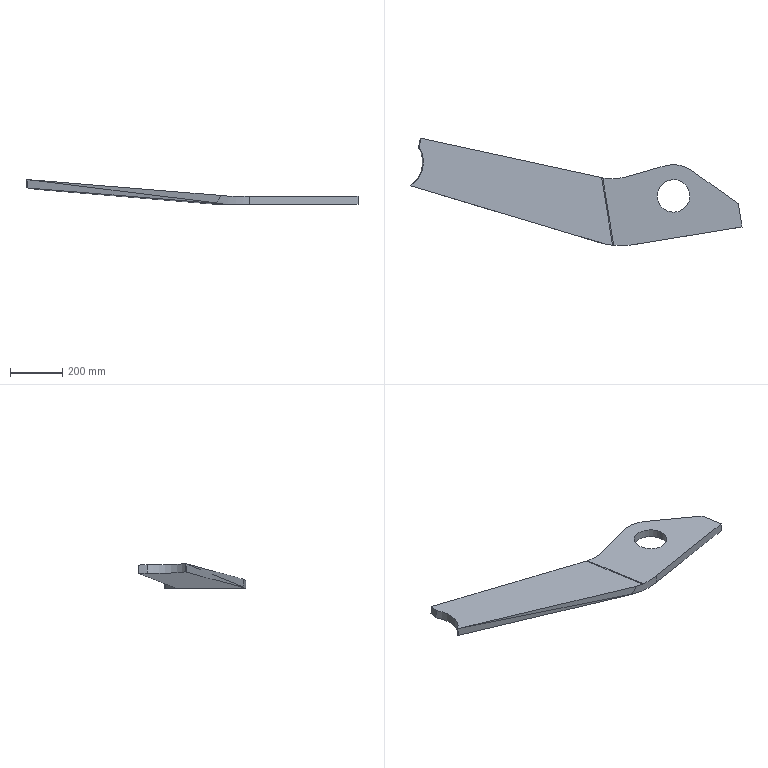Part | SolidWorks | features SplitBody 1 | 1 solid | 24 faces | box 1274 x 411.811 x 95.912 mm | volume 8557362 mm3 | plane 14 | cylinder 9 | spline 1 | commonest cylinder face diameters 125 x2 400 x2 100 x1 164 x1 220 x1 240 x1
STEP:
#1=CARTESIAN_POINT('',(4252.633,293.982,-1052.5));
#2=VERTEX_POINT('',#1);
#3=CARTESIAN_POINT('',(4129.247,273.958,-1052.5));
#4=VERTEX_POINT('',#3);
#5=CARTESIAN_POINT('',(4190.94,283.97,-1052.5));
#6=DIRECTION('',(0.,0.,-1.));
#7=DIRECTION('',(-0.9871,-0.1602,0.));
#8=AXIS2_PLACEMENT_3D('',#5,#6,#7);
#9=CIRCLE('',#8,62.5);
#10=EDGE_CURVE('',#2,#4,#9,.T.);
#11=ORIENTED_EDGE('',*,*,#10,.F.);
#12=CARTESIAN_POINT('',(4252.633,293.982,-1084.5));
#13=VERTEX_POINT('',#12);
#14=CARTESIAN_POINT('',(4252.633,293.982,-1052.5));
#15=DIRECTION('',(0.,0.,-1.));
#16=VECTOR('',#15,1000.);
#17=LINE('',#14,#16);
#18=EDGE_CURVE('',#2,#13,#17,.T.);
#19=ORIENTED_EDGE('',*,*,#18,.T.);
#20=CARTESIAN_POINT('',(4129.247,273.958,-1084.5));
#21=VERTEX_POINT('',#20);
#22=CARTESIAN_POINT('',(4190.94,283.97,-1084.5));
#23=DIRECTION('',(0.,0.,-1.));
#24=DIRECTION('',(-0.9871,-0.1602,0.));
#25=AXIS2_PLACEMENT_3D('',#22,#23,#24);
#26=CIRCLE('',#25,62.5);
#27=EDGE_CURVE('',#13,#21,#26,.T.);
#28=ORIENTED_EDGE('',*,*,#27,.T.);
#29=CARTESIAN_POINT('',(4129.247,273.958,-1052.5));
#30=DIRECTION('',(0.,0.,-1.));
#31=VECTOR('',#30,1000.);
#32=LINE('',#29,#31);
#33=EDGE_CURVE('',#4,#21,#32,.T.);
#34=ORIENTED_EDGE('',*,*,#33,.F.);
#35=EDGE_LOOP('',(#11,#19,#28,#34));
#36=FACE_OUTER_BOUND('',#35,.T.);
#37=CARTESIAN_POINT('',(4190.94,283.97,-1052.5));
#38=DIRECTION('',(0.,0.,-1.));
#39=DIRECTION('',(-0.9871,-0.1602,0.));
#40=AXIS2_PLACEMENT_3D('',#37,#38,#39);
#41=CYLINDRICAL_SURFACE('',#40,62.5);
#42=ADVANCED_FACE('',(#36),#41,.F.);
#43=CARTESIAN_POINT('',(3221.578,504.78,-994.568));
#44=VERTEX_POINT('',#43);
#45=CARTESIAN_POINT('',(3214.351,471.062,-993.471));
#46=VERTEX_POINT('',#45);
#47=CARTESIAN_POINT('',(3221.578,504.78,-994.568));
#48=DIRECTION('',(-0.2095,-0.9773,0.03179));
#49=VECTOR('',#48,1000.);
#50=LINE('',#47,#49);
#51=EDGE_CURVE('',#44,#46,#50,.T.);
#52=ORIENTED_EDGE('',*,*,#51,.T.);
#53=CARTESIAN_POINT('',(3181.855,322.901,-988.588));
#54=VERTEX_POINT('',#53);
#55=CARTESIAN_POINT('',(3120.615,414.189,-984.579));
#56=DIRECTION('',(-0.08603,-0.01396,-0.9962));
#57=DIRECTION('',(-0.9833,-0.1596,0.08716));
#58=AXIS2_PLACEMENT_3D('',#55,#56,#57);
#59=CIRCLE('',#58,110.);
#60=EDGE_CURVE('',#46,#54,#59,.T.);
#61=ORIENTED_EDGE('',*,*,#60,.T.);
#62=CARTESIAN_POINT('',(3927.771,99.208,-1049.87));
#63=VERTEX_POINT('',#62);
#64=CARTESIAN_POINT('',(3181.855,322.901,-988.588));
#65=DIRECTION('',(0.9549,-0.2864,-0.07845));
#66=VECTOR('',#65,1000.);
#67=LINE('',#64,#66);
#68=EDGE_CURVE('',#54,#63,#67,.T.);
#69=ORIENTED_EDGE('',*,*,#68,.T.);
#70=CARTESIAN_POINT('',(3956.763,94.667,-1052.31));
#71=VERTEX_POINT('',#70);
#72=CARTESIAN_POINT('',(3927.771,99.208,-1049.87));
#73=CARTESIAN_POINT('',(3937.357,97.222,-1050.67));
#74=CARTESIAN_POINT('',(3947.029,95.707,-1051.484));
#75=CARTESIAN_POINT('',(3956.763,94.667,-1052.31));
#76=(BOUNDED_CURVE()B_SPLINE_CURVE(3,(#72,#73,#74,#75),.UNSPECIFIED.,.F.,.T.)B_SPLINE_CURVE_WITH_KNOTS((4,4),(1.206,1.303),.UNSPECIFIED.)CURVE()GEOMETRIC_REPRESENTATION_ITEM()RATIONAL_B_SPLINE_CURVE((1.,0.9992,0.9992,1.))REPRESENTATION_ITEM(''));
#77=EDGE_CURVE('',#63,#71,#76,.T.);
#78=ORIENTED_EDGE('',*,*,#77,.T.);
#79=CARTESIAN_POINT('',(3914.616,354.364,-1052.31));
#80=VERTEX_POINT('',#79);
#81=CARTESIAN_POINT('',(3884.78,538.207,-1052.31));
#82=DIRECTION('',(-0.1602,0.9871,0.));
#83=VECTOR('',#82,1000.);
#84=LINE('',#81,#83);
#85=EDGE_CURVE('',#71,#80,#84,.T.);
#86=ORIENTED_EDGE('',*,*,#85,.T.);
#87=CARTESIAN_POINT('',(3914.552,354.378,-1052.304));
#88=VERTEX_POINT('',#87);
#89=CARTESIAN_POINT('',(3956.445,549.838,-1058.662));
#90=DIRECTION('',(-0.08603,-0.01396,-0.9962));
#91=DIRECTION('',(-0.9833,-0.1596,0.08716));
#92=AXIS2_PLACEMENT_3D('',#89,#90,#91);
#93=CIRCLE('',#92,200.);
#94=EDGE_CURVE('',#80,#88,#93,.T.);
#95=ORIENTED_EDGE('',*,*,#94,.T.);
#96=CARTESIAN_POINT('',(3914.552,354.378,-1052.304));
#97=DIRECTION('',(-0.974,0.2114,0.08115));
#98=VECTOR('',#97,1000.);
#99=LINE('',#96,#98);
#100=EDGE_CURVE('',#88,#44,#99,.T.);
#101=ORIENTED_EDGE('',*,*,#100,.T.);
#102=EDGE_LOOP('',(#52,#61,#69,#78,#86,#95,#101));
#103=FACE_OUTER_BOUND('',#102,.T.);
#104=CARTESIAN_POINT('',(3120.615,414.189,-984.579));
#105=DIRECTION('',(0.08603,0.01396,0.9962));
#106=DIRECTION('',(0.9833,0.1596,-0.08716));
#107=AXIS2_PLACEMENT_3D('',#104,#105,#106);
#108=PLANE('',#107);
#109=ADVANCED_FACE('',(#103),#108,.T.);
#110=CARTESIAN_POINT('',(3179.102,322.454,-1020.467));
#111=VERTEX_POINT('',#110);
#112=CARTESIAN_POINT('',(3181.855,322.901,-988.588));
#113=DIRECTION('',(-0.08603,-0.01396,-0.9962));
#114=VECTOR('',#113,1000.);
#115=LINE('',#112,#114);
#116=EDGE_CURVE('',#54,#111,#115,.T.);
#117=ORIENTED_EDGE('',*,*,#116,.F.);
#118=ORIENTED_EDGE('',*,*,#60,.F.);
#119=CARTESIAN_POINT('',(3211.598,470.615,-1025.349));
#120=VERTEX_POINT('',#119);
#121=CARTESIAN_POINT('',(3214.351,471.062,-993.471));
#122=DIRECTION('',(0.08603,0.01396,0.9962));
#123=VECTOR('',#122,1000.);
#124=LINE('',#121,#123);
#125=EDGE_CURVE('',#120,#46,#124,.T.);
#126=ORIENTED_EDGE('',*,*,#125,.F.);
#127=CARTESIAN_POINT('',(3117.862,413.742,-1016.457));
#128=DIRECTION('',(0.08603,0.01396,0.9962));
#129=DIRECTION('',(-0.9833,-0.1596,0.08716));
#130=AXIS2_PLACEMENT_3D('',#127,#128,#129);
#131=CIRCLE('',#130,110.);
#132=EDGE_CURVE('',#111,#120,#131,.T.);
#133=ORIENTED_EDGE('',*,*,#132,.F.);
#134=EDGE_LOOP('',(#117,#118,#126,#133));
#135=FACE_OUTER_BOUND('',#134,.T.);
#136=CARTESIAN_POINT('',(3120.615,414.189,-984.579));
#137=DIRECTION('',(-0.08603,-0.01396,-0.9962));
#138=DIRECTION('',(-0.9833,-0.1596,0.08716));
#139=AXIS2_PLACEMENT_3D('',#136,#137,#138);
#140=CYLINDRICAL_SURFACE('',#139,110.);
#141=ADVANCED_FACE('',(#135),#140,.F.);
#142=ORIENTED_EDGE('',*,*,#125,.T.);
#143=ORIENTED_EDGE('',*,*,#51,.F.);
#144=CARTESIAN_POINT('',(3218.825,504.333,-1026.446));
#145=VERTEX_POINT('',#144);
#146=CARTESIAN_POINT('',(3221.578,504.78,-994.568));
#147=DIRECTION('',(0.08603,0.01396,0.9962));
#148=VECTOR('',#147,1000.);
#149=LINE('',#146,#148);
#150=EDGE_CURVE('',#145,#44,#149,.T.);
#151=ORIENTED_EDGE('',*,*,#150,.F.);
#152=CARTESIAN_POINT('',(3218.825,504.333,-1026.446));
#153=DIRECTION('',(0.2095,0.9773,-0.03179));
#154=VECTOR('',#153,1000.);
#155=LINE('',#152,#154);
#156=EDGE_CURVE('',#120,#145,#155,.T.);
#157=ORIENTED_EDGE('',*,*,#156,.F.);
#158=EDGE_LOOP('',(#142,#143,#151,#157));
#159=FACE_OUTER_BOUND('',#158,.T.);
#160=CARTESIAN_POINT('',(3221.578,504.78,-994.568));
#161=DIRECTION('',(0.974,-0.2114,-0.08115));
#162=DIRECTION('',(0.2095,0.9773,-0.03179));
#163=AXIS2_PLACEMENT_3D('',#160,#161,#162);
#164=PLANE('',#163);
#165=ADVANCED_FACE('',(#159),#164,.F.);
#166=ORIENTED_EDGE('',*,*,#150,.T.);
#167=ORIENTED_EDGE('',*,*,#100,.F.);
#168=CARTESIAN_POINT('',(3911.799,353.931,-1084.183));
#169=VERTEX_POINT('',#168);
#170=CARTESIAN_POINT('',(3914.552,354.378,-1052.304));
#171=DIRECTION('',(0.08603,0.01396,0.9962));
#172=VECTOR('',#171,1000.);
#173=LINE('',#170,#172);
#174=EDGE_CURVE('',#169,#88,#173,.T.);
#175=ORIENTED_EDGE('',*,*,#174,.F.);
#176=CARTESIAN_POINT('',(3218.825,504.333,-1026.446));
#177=DIRECTION('',(0.974,-0.2114,-0.08115));
#178=VECTOR('',#177,1000.);
#179=LINE('',#176,#178);
#180=EDGE_CURVE('',#145,#169,#179,.T.);
#181=ORIENTED_EDGE('',*,*,#180,.F.);
#182=EDGE_LOOP('',(#166,#167,#175,#181));
#183=FACE_OUTER_BOUND('',#182,.T.);
#184=CARTESIAN_POINT('',(3221.578,504.78,-994.568));
#185=DIRECTION('',(-0.2095,-0.9773,0.03179));
#186=DIRECTION('',(0.974,-0.2114,-0.08115));
#187=AXIS2_PLACEMENT_3D('',#184,#185,#186);
#188=PLANE('',#187);
#189=ADVANCED_FACE('',(#183),#188,.F.);
#190=CARTESIAN_POINT('',(3961.25,94.222,-1052.5));
#191=VERTEX_POINT('',#190);
#192=CARTESIAN_POINT('',(3961.25,94.222,-1052.5));
#193=CARTESIAN_POINT('',(3959.751,94.359,-1052.5));
#194=CARTESIAN_POINT('',(3958.255,94.508,-1052.436));
#195=CARTESIAN_POINT('',(3956.763,94.667,-1052.31));
#196=B_SPLINE_CURVE_WITH_KNOTS('',3,(#192,#193,#194,#195),.UNSPECIFIED.,.F.,.F.,(4,4),(0.,0.004513),.UNSPECIFIED.);
#197=EDGE_CURVE('',#191,#71,#196,.T.);
#198=ORIENTED_EDGE('',*,*,#197,.F.);
#199=CARTESIAN_POINT('',(3919.263,352.938,-1052.5));
#200=VERTEX_POINT('',#199);
#201=CARTESIAN_POINT('',(3983.96,-45.707,-1052.5));
#202=DIRECTION('',(0.1602,-0.9871,0.));
#203=VECTOR('',#202,1000.);
#204=LINE('',#201,#203);
#205=EDGE_CURVE('',#200,#191,#204,.T.);
#206=ORIENTED_EDGE('',*,*,#205,.F.);
#207=CARTESIAN_POINT('',(3914.616,354.364,-1052.31));
#208=CARTESIAN_POINT('',(3916.162,353.888,-1052.436));
#209=CARTESIAN_POINT('',(3917.712,353.413,-1052.5));
#210=CARTESIAN_POINT('',(3919.263,352.938,-1052.5));
#211=B_SPLINE_CURVE_WITH_KNOTS('',3,(#207,#208,#209,#210),.UNSPECIFIED.,.F.,.F.,(4,4),(0.,1.),.UNSPECIFIED.);
#212=EDGE_CURVE('',#80,#200,#211,.T.);
#213=ORIENTED_EDGE('',*,*,#212,.F.);
#214=ORIENTED_EDGE('',*,*,#85,.F.);
#215=EDGE_LOOP('',(#198,#206,#213,#214));
#216=FACE_OUTER_BOUND('',#215,.T.);
#217=CARTESIAN_POINT('',(3983.96,-45.707,-1002.5));
#218=DIRECTION('',(-0.1602,0.9871,0.));
#219=DIRECTION('',(0.08603,0.01396,0.9962));
#220=AXIS2_PLACEMENT_3D('',#217,#218,#219);
#221=CYLINDRICAL_SURFACE('',#220,50.);
#222=ADVANCED_FACE('',(#216),#221,.F.);
#223=ORIENTED_EDGE('',*,*,#197,.T.);
#224=ORIENTED_EDGE('',*,*,#77,.F.);
#225=CARTESIAN_POINT('',(3902.027,105.743,-1077.67));
#226=VERTEX_POINT('',#225);
#227=CARTESIAN_POINT('',(3927.771,99.208,-1049.87));
#228=CARTESIAN_POINT('',(3919.096,101.006,-1069.446));
#229=CARTESIAN_POINT('',(3910.509,103.185,-1078.719));
#230=CARTESIAN_POINT('',(3902.027,105.743,-1077.67));
#231=(BOUNDED_CURVE()B_SPLINE_CURVE(3,(#227,#228,#229,#230),.UNSPECIFIED.,.F.,.T.)B_SPLINE_CURVE_WITH_KNOTS((4,4),(3.058,3.146),.UNSPECIFIED.)CURVE()GEOMETRIC_REPRESENTATION_ITEM()RATIONAL_B_SPLINE_CURVE((1.,0.9993,0.9993,1.))REPRESENTATION_ITEM(''));
#232=EDGE_CURVE('',#63,#226,#231,.T.);
#233=ORIENTED_EDGE('',*,*,#232,.T.);
#234=CARTESIAN_POINT('',(3902.027,105.743,-1079.86));
#235=VERTEX_POINT('',#234);
#236=CARTESIAN_POINT('',(3902.027,105.743,-1128.053));
#237=DIRECTION('',(0.,0.,-1.));
#238=VECTOR('',#237,1000.);
#239=LINE('',#236,#238);
#240=EDGE_CURVE('',#226,#235,#239,.T.);
#241=ORIENTED_EDGE('',*,*,#240,.T.);
#242=CARTESIAN_POINT('',(3953.886,94.989,-1084.188));
#243=VERTEX_POINT('',#242);
#244=CARTESIAN_POINT('',(3902.027,105.743,-1079.86));
#245=CARTESIAN_POINT('',(3918.974,100.633,-1081.252));
#246=CARTESIAN_POINT('',(3936.305,97.039,-1082.698));
#247=CARTESIAN_POINT('',(3953.886,94.989,-1084.188));
#248=(BOUNDED_CURVE()B_SPLINE_CURVE(3,(#244,#245,#246,#247),.UNSPECIFIED.,.F.,.T.)B_SPLINE_CURVE_WITH_KNOTS((4,4),(1.117,1.294),.UNSPECIFIED.)CURVE()GEOMETRIC_REPRESENTATION_ITEM()RATIONAL_B_SPLINE_CURVE((1.,0.9974,0.9974,1.))REPRESENTATION_ITEM(''));
#249=EDGE_CURVE('',#235,#243,#248,.T.);
#250=ORIENTED_EDGE('',*,*,#249,.T.);
#251=CARTESIAN_POINT('',(3961.25,94.222,-1084.5));
#252=VERTEX_POINT('',#251);
#253=CARTESIAN_POINT('',(3953.886,94.989,-1084.188));
#254=CARTESIAN_POINT('',(3956.333,94.703,-1084.395));
#255=CARTESIAN_POINT('',(3958.788,94.447,-1084.5));
#256=CARTESIAN_POINT('',(3961.25,94.222,-1084.5));
#257=B_SPLINE_CURVE_WITH_KNOTS('',3,(#253,#254,#255,#256),.UNSPECIFIED.,.F.,.F.,(4,4),(0.,0.007411),.UNSPECIFIED.);
#258=EDGE_CURVE('',#243,#252,#257,.T.);
#259=ORIENTED_EDGE('',*,*,#258,.T.);
#260=CARTESIAN_POINT('',(4036.695,96.844,-1084.5));
#261=VERTEX_POINT('',#260);
#262=CARTESIAN_POINT('',(3988.636,392.969,-1084.5));
#263=DIRECTION('',(0.,0.,1.));
#264=DIRECTION('',(0.9871,0.1602,0.));
#265=AXIS2_PLACEMENT_3D('',#262,#263,#264);
#266=CIRCLE('',#265,300.);
#267=EDGE_CURVE('',#252,#261,#266,.T.);
#268=ORIENTED_EDGE('',*,*,#267,.T.);
#269=CARTESIAN_POINT('',(4036.695,96.844,-1052.5));
#270=VERTEX_POINT('',#269);
#271=CARTESIAN_POINT('',(4036.695,96.844,-1128.053));
#272=DIRECTION('',(0.,0.,1.));
#273=VECTOR('',#272,1000.);
#274=LINE('',#271,#273);
#275=EDGE_CURVE('',#261,#270,#274,.T.);
#276=ORIENTED_EDGE('',*,*,#275,.T.);
#277=CARTESIAN_POINT('',(3988.636,392.969,-1052.5));
#278=DIRECTION('',(0.,0.,-1.));
#279=DIRECTION('',(0.9871,0.1602,0.));
#280=AXIS2_PLACEMENT_3D('',#277,#278,#279);
#281=CIRCLE('',#280,300.);
#282=EDGE_CURVE('',#270,#191,#281,.T.);
#283=ORIENTED_EDGE('',*,*,#282,.T.);
#284=EDGE_LOOP('',(#223,#224,#233,#241,#250,#259,#268,#276,#283));
#285=FACE_OUTER_BOUND('',#284,.T.);
#286=CARTESIAN_POINT('',(3988.636,392.969,-1128.053));
#287=DIRECTION('',(0.,0.,1.));
#288=DIRECTION('',(0.9871,0.1602,0.));
#289=AXIS2_PLACEMENT_3D('',#286,#287,#288);
#290=CYLINDRICAL_SURFACE('',#289,300.);
#291=ADVANCED_FACE('',(#285),#290,.T.);
#292=ORIENTED_EDGE('',*,*,#68,.F.);
#293=CARTESIAN_POINT('',(3902.027,105.743,-1077.67));
#294=DIRECTION('',(-0.9508,0.2867,0.1176));
#295=VECTOR('',#294,1000.);
#296=LINE('',#293,#295);
#297=EDGE_CURVE('',#226,#54,#296,.T.);
#298=ORIENTED_EDGE('',*,*,#297,.F.);
#299=ORIENTED_EDGE('',*,*,#232,.F.);
#300=EDGE_LOOP('',(#292,#298,#299));
#301=FACE_OUTER_BOUND('',#300,.T.);
#302=CARTESIAN_POINT('',(3181.855,322.901,-988.588));
#303=DIRECTION('',(0.2842,0.958,-0.03797));
#304=DIRECTION('',(-0.9549,0.2864,0.07845));
#305=AXIS2_PLACEMENT_3D('',#302,#303,#304);
#306=PLANE('',#305);
#307=ADVANCED_FACE('',(#301),#306,.F.);
#308=CARTESIAN_POINT('',(3181.855,322.901,-1020.711));
#309=VERTEX_POINT('',#308);
#310=CARTESIAN_POINT('',(3181.855,322.901,-1020.711));
#311=DIRECTION('',(0.9545,-0.2878,-0.07839));
#312=VECTOR('',#311,1000.);
#313=LINE('',#310,#312);
#314=EDGE_CURVE('',#309,#235,#313,.T.);
#315=ORIENTED_EDGE('',*,*,#314,.F.);
#316=CARTESIAN_POINT('',(3186.707,320.173,-1021.091));
#317=VERTEX_POINT('',#316);
#318=CARTESIAN_POINT('',(3186.707,320.173,-1021.091));
#319=DIRECTION('',(-0.8697,0.4889,0.06825));
#320=VECTOR('',#319,1000.);
#321=LINE('',#318,#320);
#322=EDGE_CURVE('',#317,#309,#321,.T.);
#323=ORIENTED_EDGE('',*,*,#322,.F.);
#324=CARTESIAN_POINT('',(3179.102,322.454,-1020.467));
#325=DIRECTION('',(0.9549,-0.2864,-0.07845));
#326=VECTOR('',#325,1000.);
#327=LINE('',#324,#326);
#328=EDGE_CURVE('',#111,#317,#327,.T.);
#329=ORIENTED_EDGE('',*,*,#328,.F.);
#330=ORIENTED_EDGE('',*,*,#132,.T.);
#331=ORIENTED_EDGE('',*,*,#156,.T.);
#332=ORIENTED_EDGE('',*,*,#180,.T.);
#333=CARTESIAN_POINT('',(3911.863,353.917,-1084.188));
#334=VERTEX_POINT('',#333);
#335=CARTESIAN_POINT('',(3911.863,353.917,-1084.188));
#336=DIRECTION('',(-0.9741,0.2112,0.08116));
#337=VECTOR('',#336,1000.);
#338=LINE('',#335,#337);
#339=EDGE_CURVE('',#334,#169,#338,.T.);
#340=ORIENTED_EDGE('',*,*,#339,.F.);
#341=CARTESIAN_POINT('',(3882.027,537.761,-1084.188));
#342=DIRECTION('',(-0.1602,0.9871,0.));
#343=VECTOR('',#342,1000.);
#344=LINE('',#341,#343);
#345=EDGE_CURVE('',#243,#334,#344,.T.);
#346=ORIENTED_EDGE('',*,*,#345,.F.);
#347=ORIENTED_EDGE('',*,*,#249,.F.);
#348=EDGE_LOOP('',(#315,#323,#329,#330,#331,#332,#340,#346,#347));
#349=FACE_OUTER_BOUND('',#348,.T.);
#350=CARTESIAN_POINT('',(3117.862,413.742,-1016.457));
#351=DIRECTION('',(0.08603,0.01396,0.9962));
#352=DIRECTION('',(0.9833,0.1596,-0.08716));
#353=AXIS2_PLACEMENT_3D('',#350,#351,#352);
#354=PLANE('',#353);
#355=ADVANCED_FACE('',(#349),#354,.F.);
#356=CARTESIAN_POINT('',(3181.855,322.901,-988.588));
#357=DIRECTION('',(0.1471,-0.08271,-0.9857));
#358=VECTOR('',#357,1000.);
#359=LINE('',#356,#358);
#360=EDGE_CURVE('',#54,#317,#359,.T.);
#361=ORIENTED_EDGE('',*,*,#360,.F.);
#362=ORIENTED_EDGE('',*,*,#116,.T.);
#363=ORIENTED_EDGE('',*,*,#328,.T.);
#364=EDGE_LOOP('',(#361,#362,#363));
#365=FACE_OUTER_BOUND('',#364,.T.);
#366=CARTESIAN_POINT('',(3181.855,322.901,-988.588));
#367=DIRECTION('',(0.2842,0.958,-0.03797));
#368=DIRECTION('',(-0.9549,0.2864,0.07845));
#369=AXIS2_PLACEMENT_3D('',#366,#367,#368);
#370=PLANE('',#369);
#371=ADVANCED_FACE('',(#365),#370,.F.);
#372=CARTESIAN_POINT('',(3914.616,354.364,-1052.31));
#373=DIRECTION('',(0.08603,0.01396,0.9962));
#374=VECTOR('',#373,1000.);
#375=LINE('',#372,#374);
#376=EDGE_CURVE('',#334,#80,#375,.T.);
#377=ORIENTED_EDGE('',*,*,#376,.F.);
#378=ORIENTED_EDGE('',*,*,#339,.T.);
#379=ORIENTED_EDGE('',*,*,#174,.T.);
#380=ORIENTED_EDGE('',*,*,#94,.F.);
#381=EDGE_LOOP('',(#377,#378,#379,#380));
#382=FACE_OUTER_BOUND('',#381,.T.);
#383=CARTESIAN_POINT('',(3956.445,549.838,-1058.662));
#384=DIRECTION('',(-0.08603,-0.01396,-0.9962));
#385=DIRECTION('',(-0.9833,-0.1596,0.08716));
#386=AXIS2_PLACEMENT_3D('',#383,#384,#385);
#387=CYLINDRICAL_SURFACE('',#386,200.);
#388=ADVANCED_FACE('',(#382),#387,.F.);
#389=CARTESIAN_POINT('',(4158.117,399.394,-1052.5));
#390=VERTEX_POINT('',#389);
#391=CARTESIAN_POINT('',(4010.04,357.285,-1052.5));
#392=VERTEX_POINT('',#391);
#393=CARTESIAN_POINT('',(4158.117,399.394,-1052.5));
#394=DIRECTION('',(-0.9619,-0.2735,0.));
#395=VECTOR('',#394,1000.);
#396=LINE('',#393,#395);
#397=EDGE_CURVE('',#390,#392,#396,.T.);
#398=ORIENTED_EDGE('',*,*,#397,.T.);
#399=CARTESIAN_POINT('',(3955.335,549.658,-1052.5));
#400=DIRECTION('',(0.,0.,-1.));
#401=DIRECTION('',(-0.9871,-0.1602,0.));
#402=AXIS2_PLACEMENT_3D('',#399,#400,#401);
#403=CIRCLE('',#402,200.);
#404=EDGE_CURVE('',#392,#200,#403,.T.);
#405=ORIENTED_EDGE('',*,*,#404,.T.);
#406=ORIENTED_EDGE('',*,*,#205,.T.);
#407=ORIENTED_EDGE('',*,*,#282,.F.);
#408=CARTESIAN_POINT('',(4453.472,164.483,-1052.5));
#409=VERTEX_POINT('',#408);
#410=CARTESIAN_POINT('',(3190.003,-40.568,-1052.5));
#411=DIRECTION('',(0.9871,0.1602,0.));
#412=VECTOR('',#411,1000.);
#413=LINE('',#410,#412);
#414=EDGE_CURVE('',#270,#409,#413,.T.);
#415=ORIENTED_EDGE('',*,*,#414,.T.);
#416=CARTESIAN_POINT('',(4439.054,253.321,-1052.5));
#417=VERTEX_POINT('',#416);
#418=CARTESIAN_POINT('',(4379.781,618.543,-1052.5));
#419=DIRECTION('',(-0.1602,0.9871,0.));
#420=VECTOR('',#419,1000.);
#421=LINE('',#418,#420);
#422=EDGE_CURVE('',#409,#417,#421,.T.);
#423=ORIENTED_EDGE('',*,*,#422,.T.);
#424=CARTESIAN_POINT('',(4261.011,381.386,-1052.5));
#425=VERTEX_POINT('',#424);
#426=CARTESIAN_POINT('',(4439.054,253.321,-1052.5));
#427=DIRECTION('',(-0.8118,0.5839,0.));
#428=VECTOR('',#427,1000.);
#429=LINE('',#426,#428);
#430=EDGE_CURVE('',#417,#425,#429,.T.);
#431=ORIENTED_EDGE('',*,*,#430,.T.);
#432=CARTESIAN_POINT('',(4190.94,283.97,-1052.5));
#433=DIRECTION('',(0.,0.,1.));
#434=DIRECTION('',(-0.9871,-0.1602,0.));
#435=AXIS2_PLACEMENT_3D('',#432,#433,#434);
#436=CIRCLE('',#435,120.);
#437=EDGE_CURVE('',#425,#390,#436,.T.);
#438=ORIENTED_EDGE('',*,*,#437,.T.);
#439=EDGE_LOOP('',(#398,#405,#406,#407,#415,#423,#431,#438));
#440=FACE_OUTER_BOUND('',#439,.T.);
#441=CARTESIAN_POINT('',(4190.94,283.97,-1052.5));
#442=DIRECTION('',(0.,0.,-1.));
#443=DIRECTION('',(-0.9871,-0.1602,0.));
#444=AXIS2_PLACEMENT_3D('',#441,#442,#443);
#445=CIRCLE('',#444,62.5);
#446=EDGE_CURVE('',#4,#2,#445,.T.);
#447=ORIENTED_EDGE('',*,*,#446,.T.);
#448=ORIENTED_EDGE('',*,*,#10,.T.);
#449=EDGE_LOOP('',(#447,#448));
#450=FACE_BOUND('',#449,.T.);
#451=CARTESIAN_POINT('',(3116.313,413.491,-1052.5));
#452=DIRECTION('',(0.,0.,1.));
#453=DIRECTION('',(0.9871,0.1602,0.));
#454=AXIS2_PLACEMENT_3D('',#451,#452,#453);
#455=PLANE('',#454);
#456=ADVANCED_FACE('',(#440,#450),#455,.T.);
#457=CARTESIAN_POINT('',(3919.263,352.938,-1084.5));
#458=VERTEX_POINT('',#457);
#459=CARTESIAN_POINT('',(3911.863,353.917,-1084.188));
#460=CARTESIAN_POINT('',(3914.324,353.59,-1084.396));
#461=CARTESIAN_POINT('',(3916.793,353.264,-1084.5));
#462=CARTESIAN_POINT('',(3919.263,352.938,-1084.5));
#463=B_SPLINE_CURVE_WITH_KNOTS('',3,(#459,#460,#461,#462),.UNSPECIFIED.,.F.,.F.,(4,4),(0.,1.),.UNSPECIFIED.);
#464=EDGE_CURVE('',#334,#458,#463,.T.);
#465=ORIENTED_EDGE('',*,*,#464,.F.);
#466=ORIENTED_EDGE('',*,*,#376,.T.);
#467=ORIENTED_EDGE('',*,*,#212,.T.);
#468=CARTESIAN_POINT('',(3919.263,352.938,-1068.5));
#469=DIRECTION('',(0.,0.,1.));
#470=VECTOR('',#469,1000.);
#471=LINE('',#468,#470);
#472=EDGE_CURVE('',#458,#200,#471,.T.);
#473=ORIENTED_EDGE('',*,*,#472,.F.);
#474=EDGE_LOOP('',(#465,#466,#467,#473));
#475=FACE_OUTER_BOUND('',#474,.T.);
#476=CARTESIAN_POINT('',(3919.263,352.938,-1084.82));
#477=CARTESIAN_POINT('',(3916.784,353.262,-1084.82));
#478=CARTESIAN_POINT('',(3914.306,353.587,-1084.715));
#479=CARTESIAN_POINT('',(3911.836,353.913,-1084.507));
#480=CARTESIAN_POINT('',(3919.263,352.938,-1084.5));
#481=CARTESIAN_POINT('',(3916.793,353.264,-1084.5));
#482=CARTESIAN_POINT('',(3914.324,353.59,-1084.396));
#483=CARTESIAN_POINT('',(3911.863,353.917,-1084.188));
#484=CARTESIAN_POINT('',(3919.263,352.938,-1052.5));
#485=CARTESIAN_POINT('',(3917.712,353.413,-1052.5));
#486=CARTESIAN_POINT('',(3916.162,353.888,-1052.436));
#487=CARTESIAN_POINT('',(3914.616,354.364,-1052.31));
#488=B_SPLINE_SURFACE_WITH_KNOTS('',1,3,((#476,#477,#478,#479),(#480,#481,#482,#483),(#484,#485,#486,#487)),.UNSPECIFIED.,.F.,.F.,.F.,(2,1,2),(4,4),(-0.01,0.,1.),(0.,1.),.UNSPECIFIED.);
#489=ADVANCED_FACE('',(#475),#488,.F.);
#490=CARTESIAN_POINT('',(4453.472,164.483,-1084.5));
#491=VERTEX_POINT('',#490);
#492=CARTESIAN_POINT('',(4453.472,164.483,-1084.5));
#493=DIRECTION('',(-0.9871,-0.1602,0.));
#494=VECTOR('',#493,1000.);
#495=LINE('',#492,#494);
#496=EDGE_CURVE('',#491,#261,#495,.T.);
#497=ORIENTED_EDGE('',*,*,#496,.F.);
#498=CARTESIAN_POINT('',(4453.472,164.483,-1052.5));
#499=DIRECTION('',(0.,0.,-1.));
#500=VECTOR('',#499,1000.);
#501=LINE('',#498,#500);
#502=EDGE_CURVE('',#409,#491,#501,.T.);
#503=ORIENTED_EDGE('',*,*,#502,.F.);
#504=ORIENTED_EDGE('',*,*,#414,.F.);
#505=ORIENTED_EDGE('',*,*,#275,.F.);
#506=EDGE_LOOP('',(#497,#503,#504,#505));
#507=FACE_OUTER_BOUND('',#506,.T.);
#508=CARTESIAN_POINT('',(3969.8,85.987,-1052.5));
#509=DIRECTION('',(-0.1602,0.9871,0.));
#510=DIRECTION('',(0.08603,0.01396,0.9962));
#511=AXIS2_PLACEMENT_3D('',#508,#509,#510);
#512=PLANE('',#511);
#513=ADVANCED_FACE('',(#507),#512,.F.);
#514=CARTESIAN_POINT('',(3889.082,538.906,-1084.5));
#515=DIRECTION('',(0.1602,-0.9871,0.));
#516=VECTOR('',#515,1000.);
#517=LINE('',#514,#516);
#518=EDGE_CURVE('',#458,#252,#517,.T.);
#519=ORIENTED_EDGE('',*,*,#518,.F.);
#520=CARTESIAN_POINT('',(4010.04,357.285,-1084.5));
#521=VERTEX_POINT('',#520);
#522=CARTESIAN_POINT('',(3955.335,549.658,-1084.5));
#523=DIRECTION('',(0.,0.,-1.));
#524=DIRECTION('',(-0.9871,-0.1602,0.));
#525=AXIS2_PLACEMENT_3D('',#522,#523,#524);
#526=CIRCLE('',#525,200.);
#527=EDGE_CURVE('',#521,#458,#526,.T.);
#528=ORIENTED_EDGE('',*,*,#527,.F.);
#529=CARTESIAN_POINT('',(4158.117,399.394,-1084.5));
#530=VERTEX_POINT('',#529);
#531=CARTESIAN_POINT('',(4158.117,399.394,-1084.5));
#532=DIRECTION('',(-0.9619,-0.2735,0.));
#533=VECTOR('',#532,1000.);
#534=LINE('',#531,#533);
#535=EDGE_CURVE('',#530,#521,#534,.T.);
#536=ORIENTED_EDGE('',*,*,#535,.F.);
#537=CARTESIAN_POINT('',(4261.011,381.386,-1084.5));
#538=VERTEX_POINT('',#537);
#539=CARTESIAN_POINT('',(4190.94,283.97,-1084.5));
#540=DIRECTION('',(0.,0.,1.));
#541=DIRECTION('',(-0.9871,-0.1602,0.));
#542=AXIS2_PLACEMENT_3D('',#539,#540,#541);
#543=CIRCLE('',#542,120.);
#544=EDGE_CURVE('',#538,#530,#543,.T.);
#545=ORIENTED_EDGE('',*,*,#544,.F.);
#546=CARTESIAN_POINT('',(4439.054,253.321,-1084.5));
#547=VERTEX_POINT('',#546);
#548=CARTESIAN_POINT('',(4439.054,253.321,-1084.5));
#549=DIRECTION('',(-0.8118,0.5839,0.));
#550=VECTOR('',#549,1000.);
#551=LINE('',#548,#550);
#552=EDGE_CURVE('',#547,#538,#551,.T.);
#553=ORIENTED_EDGE('',*,*,#552,.F.);
#554=CARTESIAN_POINT('',(4379.781,618.543,-1084.5));
#555=DIRECTION('',(-0.1602,0.9871,0.));
#556=VECTOR('',#555,1000.);
#557=LINE('',#554,#556);
#558=EDGE_CURVE('',#491,#547,#557,.T.);
#559=ORIENTED_EDGE('',*,*,#558,.F.);
#560=ORIENTED_EDGE('',*,*,#496,.T.);
#561=ORIENTED_EDGE('',*,*,#267,.F.);
#562=EDGE_LOOP('',(#519,#528,#536,#545,#553,#559,#560,#561));
#563=FACE_OUTER_BOUND('',#562,.T.);
#564=CARTESIAN_POINT('',(4190.94,283.97,-1084.5));
#565=DIRECTION('',(0.,0.,-1.));
#566=DIRECTION('',(-0.9871,-0.1602,0.));
#567=AXIS2_PLACEMENT_3D('',#564,#565,#566);
#568=CIRCLE('',#567,62.5);
#569=EDGE_CURVE('',#21,#13,#568,.T.);
#570=ORIENTED_EDGE('',*,*,#569,.F.);
#571=ORIENTED_EDGE('',*,*,#27,.F.);
#572=EDGE_LOOP('',(#570,#571));
#573=FACE_BOUND('',#572,.T.);
#574=CARTESIAN_POINT('',(3116.313,413.491,-1084.5));
#575=DIRECTION('',(0.,0.,1.));
#576=DIRECTION('',(0.9871,0.1602,0.));
#577=AXIS2_PLACEMENT_3D('',#574,#575,#576);
#578=PLANE('',#577);
#579=ADVANCED_FACE('',(#563,#573),#578,.F.);
#580=ORIENTED_EDGE('',*,*,#464,.T.);
#581=ORIENTED_EDGE('',*,*,#518,.T.);
#582=ORIENTED_EDGE('',*,*,#258,.F.);
#583=ORIENTED_EDGE('',*,*,#345,.T.);
#584=EDGE_LOOP('',(#580,#581,#582,#583));
#585=FACE_OUTER_BOUND('',#584,.T.);
#586=CARTESIAN_POINT('',(3983.96,-45.707,-1002.5));
#587=DIRECTION('',(-0.1602,0.9871,0.));
#588=DIRECTION('',(0.08603,0.01396,0.9962));
#589=AXIS2_PLACEMENT_3D('',#586,#587,#588);
#590=CYLINDRICAL_SURFACE('',#589,82.);
#591=ADVANCED_FACE('',(#585),#590,.T.);
#592=ORIENTED_EDGE('',*,*,#297,.T.);
#593=CARTESIAN_POINT('',(3181.855,322.901,-988.588));
#594=DIRECTION('',(0.,0.,-1.));
#595=VECTOR('',#594,1000.);
#596=LINE('',#593,#595);
#597=EDGE_CURVE('',#54,#309,#596,.T.);
#598=ORIENTED_EDGE('',*,*,#597,.T.);
#599=ORIENTED_EDGE('',*,*,#314,.T.);
#600=ORIENTED_EDGE('',*,*,#240,.F.);
#601=EDGE_LOOP('',(#592,#598,#599,#600));
#602=FACE_OUTER_BOUND('',#601,.T.);
#603=CARTESIAN_POINT('',(4253.601,-0.2692,-1128.053));
#604=DIRECTION('',(-0.2887,-0.9574,0.));
#605=DIRECTION('',(0.9545,-0.2878,-0.07839));
#606=AXIS2_PLACEMENT_3D('',#603,#604,#605);
#607=PLANE('',#606);
#608=ADVANCED_FACE('',(#602),#607,.T.);
#609=ORIENTED_EDGE('',*,*,#360,.T.);
#610=ORIENTED_EDGE('',*,*,#322,.T.);
#611=ORIENTED_EDGE('',*,*,#597,.F.);
#612=EDGE_LOOP('',(#609,#610,#611));
#613=FACE_OUTER_BOUND('',#612,.T.);
#614=CARTESIAN_POINT('',(4304.368,-308.1,-1128.053));
#615=DIRECTION('',(-0.49,-0.8717,0.));
#616=DIRECTION('',(0.8697,-0.4889,-0.06825));
#617=AXIS2_PLACEMENT_3D('',#614,#615,#616);
#618=PLANE('',#617);
#619=ADVANCED_FACE('',(#613),#618,.F.);
#620=ORIENTED_EDGE('',*,*,#404,.F.);
#621=CARTESIAN_POINT('',(4010.04,357.285,-1052.5));
#622=DIRECTION('',(0.,0.,1.));
#623=VECTOR('',#622,1000.);
#624=LINE('',#621,#623);
#625=EDGE_CURVE('',#521,#392,#624,.T.);
#626=ORIENTED_EDGE('',*,*,#625,.F.);
#627=ORIENTED_EDGE('',*,*,#527,.T.);
#628=ORIENTED_EDGE('',*,*,#472,.T.);
#629=EDGE_LOOP('',(#620,#626,#627,#628));
#630=FACE_OUTER_BOUND('',#629,.T.);
#631=CARTESIAN_POINT('',(3955.335,549.658,-1052.5));
#632=DIRECTION('',(0.,0.,-1.));
#633=DIRECTION('',(-0.9871,-0.1602,0.));
#634=AXIS2_PLACEMENT_3D('',#631,#632,#633);
#635=CYLINDRICAL_SURFACE('',#634,200.);
#636=ADVANCED_FACE('',(#630),#635,.F.);
#637=ORIENTED_EDGE('',*,*,#625,.T.);
#638=ORIENTED_EDGE('',*,*,#397,.F.);
#639=CARTESIAN_POINT('',(4158.117,399.394,-1084.5));
#640=DIRECTION('',(0.,0.,1.));
#641=VECTOR('',#640,1000.);
#642=LINE('',#639,#641);
#643=EDGE_CURVE('',#530,#390,#642,.T.);
#644=ORIENTED_EDGE('',*,*,#643,.F.);
#645=ORIENTED_EDGE('',*,*,#535,.T.);
#646=EDGE_LOOP('',(#637,#638,#644,#645));
#647=FACE_OUTER_BOUND('',#646,.T.);
#648=CARTESIAN_POINT('',(4158.117,399.394,-1052.5));
#649=DIRECTION('',(0.2735,-0.9619,0.));
#650=DIRECTION('',(0.9583,0.2725,-0.08657));
#651=AXIS2_PLACEMENT_3D('',#648,#649,#650);
#652=PLANE('',#651);
#653=ADVANCED_FACE('',(#647),#652,.F.);
#654=ORIENTED_EDGE('',*,*,#437,.F.);
#655=CARTESIAN_POINT('',(4261.011,381.386,-1052.5));
#656=DIRECTION('',(0.,0.,-1.));
#657=VECTOR('',#656,1000.);
#658=LINE('',#655,#657);
#659=EDGE_CURVE('',#425,#538,#658,.T.);
#660=ORIENTED_EDGE('',*,*,#659,.T.);
#661=ORIENTED_EDGE('',*,*,#544,.T.);
#662=ORIENTED_EDGE('',*,*,#643,.T.);
#663=EDGE_LOOP('',(#654,#660,#661,#662));
#664=FACE_OUTER_BOUND('',#663,.T.);
#665=CARTESIAN_POINT('',(4190.94,283.97,-1052.5));
#666=DIRECTION('',(0.,0.,-1.));
#667=DIRECTION('',(-0.9871,-0.1602,0.));
#668=AXIS2_PLACEMENT_3D('',#665,#666,#667);
#669=CYLINDRICAL_SURFACE('',#668,120.);
#670=ADVANCED_FACE('',(#664),#669,.T.);
#671=ORIENTED_EDGE('',*,*,#659,.F.);
#672=ORIENTED_EDGE('',*,*,#430,.F.);
#673=CARTESIAN_POINT('',(4439.054,253.321,-1084.5));
#674=DIRECTION('',(0.,0.,1.));
#675=VECTOR('',#674,1000.);
#676=LINE('',#673,#675);
#677=EDGE_CURVE('',#547,#417,#676,.T.);
#678=ORIENTED_EDGE('',*,*,#677,.F.);
#679=ORIENTED_EDGE('',*,*,#552,.T.);
#680=EDGE_LOOP('',(#671,#672,#678,#679));
#681=FACE_OUTER_BOUND('',#680,.T.);
#682=CARTESIAN_POINT('',(4439.054,253.321,-1052.5));
#683=DIRECTION('',(-0.5839,-0.8118,0.));
#684=DIRECTION('',(0.8103,-0.5828,-0.0618));
#685=AXIS2_PLACEMENT_3D('',#682,#683,#684);
#686=PLANE('',#685);
#687=ADVANCED_FACE('',(#681),#686,.F.);
#688=ORIENTED_EDGE('',*,*,#677,.T.);
#689=ORIENTED_EDGE('',*,*,#422,.F.);
#690=ORIENTED_EDGE('',*,*,#502,.T.);
#691=ORIENTED_EDGE('',*,*,#558,.T.);
#692=EDGE_LOOP('',(#688,#689,#690,#691));
#693=FACE_OUTER_BOUND('',#692,.T.);
#694=CARTESIAN_POINT('',(4453.472,164.483,-1052.5));
#695=DIRECTION('',(-0.9871,-0.1602,0.));
#696=DIRECTION('',(0.,0.,1.));
#697=AXIS2_PLACEMENT_3D('',#694,#695,#696);
#698=PLANE('',#697);
#699=ADVANCED_FACE('',(#693),#698,.F.);
#700=ORIENTED_EDGE('',*,*,#18,.F.);
#701=ORIENTED_EDGE('',*,*,#446,.F.);
#702=ORIENTED_EDGE('',*,*,#33,.T.);
#703=ORIENTED_EDGE('',*,*,#569,.T.);
#704=EDGE_LOOP('',(#700,#701,#702,#703));
#705=FACE_OUTER_BOUND('',#704,.T.);
#706=CARTESIAN_POINT('',(4190.94,283.97,-1052.5));
#707=DIRECTION('',(0.,0.,-1.));
#708=DIRECTION('',(-0.9871,-0.1602,0.));
#709=AXIS2_PLACEMENT_3D('',#706,#707,#708);
#710=CYLINDRICAL_SURFACE('',#709,62.5);
#711=ADVANCED_FACE('',(#705),#710,.F.);
#712=CLOSED_SHELL('',(#42,#109,#141,#165,#189,#222,#291,#307,#355,#371,#388,#456,#489,#513,#579,#591,#608,#619,#636,#653,#670,#687,#699,#711));
#713=MANIFOLD_SOLID_BREP('',#712);
#714=CARTESIAN_POINT('',(0.,0.,0.));
#715=DIRECTION('',(0.,0.,1.));
#716=DIRECTION('',(1.,0.,0.));
#717=AXIS2_PLACEMENT_3D('',#714,#715,#716);
#718=(LENGTH_UNIT()NAMED_UNIT(*)SI_UNIT(.MILLI.,.METRE.));
#719=UNCERTAINTY_MEASURE_WITH_UNIT(LENGTH_MEASURE(0.00001),#718,'','');
#720=(NAMED_UNIT(*)PLANE_ANGLE_UNIT()SI_UNIT($,.RADIAN.));
#721=(NAMED_UNIT(*)SI_UNIT($,.STERADIAN.)SOLID_ANGLE_UNIT());
#722=(GEOMETRIC_REPRESENTATION_CONTEXT(3)GLOBAL_UNCERTAINTY_ASSIGNED_CONTEXT((#719))GLOBAL_UNIT_ASSIGNED_CONTEXT((#718,#720,#721))REPRESENTATION_CONTEXT('',''));
#723=ADVANCED_BREP_SHAPE_REPRESENTATION('',(#713,#717),#722);